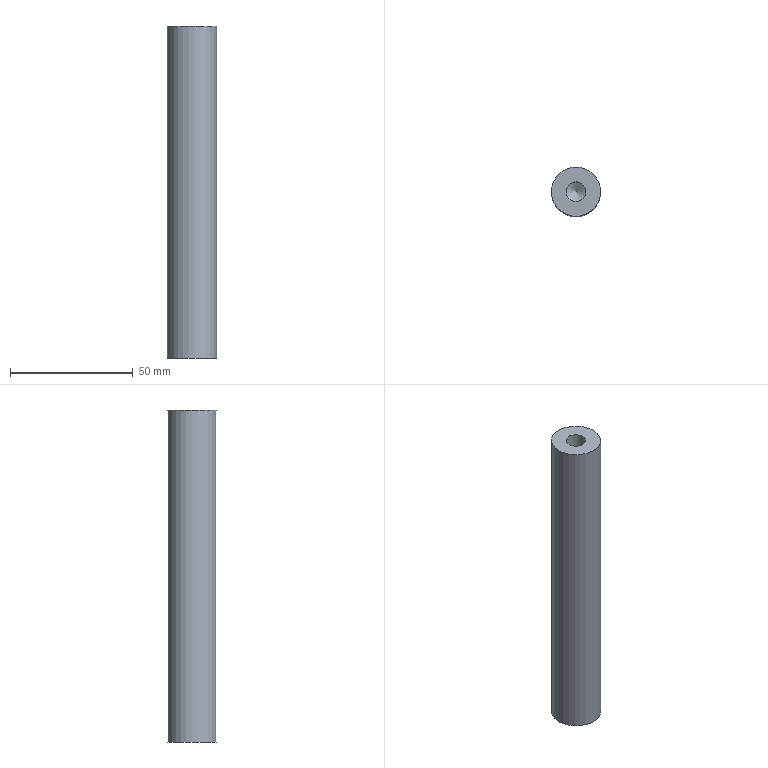Part | NX | features solid 2 | 1 solid | 7 faces | box 20 x 20 x 135 mm | volume 38516 mm3 | cylinder 3 | plane 2 | cone 2 | commonest cylinder face diameters 8 x1 12 x1 20 x1
STEP:
#1=CARTESIAN_POINT('',(-10.,175.,-155.));
#2=VERTEX_POINT('',#1);
#3=CARTESIAN_POINT('',(0.,175.,-155.));
#4=DIRECTION('',(0.,0.,-1.));
#5=DIRECTION('',(-1.,0.,0.));
#6=AXIS2_PLACEMENT_3D('',#3,#4,#5);
#7=CIRCLE('',#6,10.);
#8=EDGE_CURVE('',#2,#2,#7,.T.);
#9=ORIENTED_EDGE('',*,*,#8,.F.);
#10=EDGE_LOOP('',(#9));
#11=FACE_BOUND('',#10,.T.);
#12=CARTESIAN_POINT('',(10.,175.,-20.));
#13=VERTEX_POINT('',#12);
#14=CARTESIAN_POINT('',(0.,175.,-20.));
#15=DIRECTION('',(0.,0.,1.));
#16=DIRECTION('',(1.,0.,0.));
#17=AXIS2_PLACEMENT_3D('',#14,#15,#16);
#18=CIRCLE('',#17,10.);
#19=EDGE_CURVE('',#13,#13,#18,.F.);
#20=ORIENTED_EDGE('',*,*,#19,.T.);
#21=EDGE_LOOP('',(#20));
#22=FACE_BOUND('',#21,.T.);
#23=CARTESIAN_POINT('',(0.,175.,-97.));
#24=DIRECTION('',(0.,0.,1.));
#25=DIRECTION('',(0.,1.,0.));
#26=AXIS2_PLACEMENT_3D('',#23,#24,#25);
#27=CYLINDRICAL_SURFACE('',#26,10.);
#28=ADVANCED_FACE('',(#11,#22),#27,.T.);
#29=CARTESIAN_POINT('',(-6.,175.,-155.));
#30=VERTEX_POINT('',#29);
#31=CARTESIAN_POINT('',(0.,175.,-155.));
#32=DIRECTION('',(0.,0.,1.));
#33=DIRECTION('',(-1.,0.,0.));
#34=AXIS2_PLACEMENT_3D('',#31,#32,#33);
#35=CIRCLE('',#34,6.);
#36=EDGE_CURVE('',#30,#30,#35,.T.);
#37=ORIENTED_EDGE('',*,*,#36,.T.);
#38=EDGE_LOOP('',(#37));
#39=FACE_BOUND('',#38,.T.);
#40=ORIENTED_EDGE('',*,*,#8,.T.);
#41=EDGE_LOOP('',(#40));
#42=FACE_BOUND('',#41,.T.);
#43=CARTESIAN_POINT('',(0.,175.,-155.));
#44=DIRECTION('',(0.,0.,-1.));
#45=DIRECTION('',(0.,-1.,0.));
#46=AXIS2_PLACEMENT_3D('',#43,#44,#45);
#47=PLANE('',#46);
#48=ADVANCED_FACE('',(#39,#42),#47,.T.);
#49=CARTESIAN_POINT('',(-6.,175.,-131.));
#50=VERTEX_POINT('',#49);
#51=CARTESIAN_POINT('',(0.,175.,-131.));
#52=DIRECTION('',(0.,0.,1.));
#53=DIRECTION('',(-1.,0.,0.));
#54=AXIS2_PLACEMENT_3D('',#51,#52,#53);
#55=CIRCLE('',#54,6.);
#56=EDGE_CURVE('',#50,#50,#55,.T.);
#57=ORIENTED_EDGE('',*,*,#56,.F.);
#58=EDGE_LOOP('',(#57));
#59=FACE_BOUND('',#58,.T.);
#60=CARTESIAN_POINT('',(0.,175.,-127.395));
#61=VERTEX_POINT('',#60);
#62=VERTEX_LOOP('',#61);
#63=FACE_BOUND('',#62,.T.);
#64=CARTESIAN_POINT('',(0.,175.,-131.));
#65=DIRECTION('',(0.,0.,-1.));
#66=DIRECTION('',(1.,0.,0.));
#67=AXIS2_PLACEMENT_3D('',#64,#65,#66);
#68=CONICAL_SURFACE('',#67,6.,1.03);
#69=ADVANCED_FACE('',(#59,#63),#68,.F.);
#70=ORIENTED_EDGE('',*,*,#56,.T.);
#71=EDGE_LOOP('',(#70));
#72=FACE_BOUND('',#71,.T.);
#73=ORIENTED_EDGE('',*,*,#36,.F.);
#74=EDGE_LOOP('',(#73));
#75=FACE_BOUND('',#74,.T.);
#76=CARTESIAN_POINT('',(0.,175.,-145.));
#77=DIRECTION('',(0.,0.,1.));
#78=DIRECTION('',(-1.,0.,0.));
#79=AXIS2_PLACEMENT_3D('',#76,#77,#78);
#80=CYLINDRICAL_SURFACE('',#79,6.);
#81=ADVANCED_FACE('',(#72,#75),#80,.F.);
#82=CARTESIAN_POINT('',(-4.,175.,-20.));
#83=VERTEX_POINT('',#82);
#84=CARTESIAN_POINT('',(0.,175.,-20.));
#85=DIRECTION('',(0.,0.,-1.));
#86=DIRECTION('',(-1.,0.,0.));
#87=AXIS2_PLACEMENT_3D('',#84,#85,#86);
#88=CIRCLE('',#87,4.);
#89=EDGE_CURVE('',#83,#83,#88,.T.);
#90=ORIENTED_EDGE('',*,*,#89,.T.);
#91=EDGE_LOOP('',(#90));
#92=FACE_BOUND('',#91,.T.);
#93=ORIENTED_EDGE('',*,*,#19,.F.);
#94=EDGE_LOOP('',(#93));
#95=FACE_BOUND('',#94,.T.);
#96=CARTESIAN_POINT('',(0.,175.,-20.));
#97=DIRECTION('',(0.,0.,1.));
#98=DIRECTION('',(1.,0.,0.));
#99=AXIS2_PLACEMENT_3D('',#96,#97,#98);
#100=PLANE('',#99);
#101=ADVANCED_FACE('',(#92,#95),#100,.T.);
#102=CARTESIAN_POINT('',(-4.,175.,-40.));
#103=VERTEX_POINT('',#102);
#104=CARTESIAN_POINT('',(0.,175.,-40.));
#105=DIRECTION('',(0.,0.,-1.));
#106=DIRECTION('',(-1.,0.,0.));
#107=AXIS2_PLACEMENT_3D('',#104,#105,#106);
#108=CIRCLE('',#107,4.);
#109=EDGE_CURVE('',#103,#103,#108,.T.);
#110=ORIENTED_EDGE('',*,*,#109,.F.);
#111=EDGE_LOOP('',(#110));
#112=FACE_BOUND('',#111,.T.);
#113=CARTESIAN_POINT('',(0.,175.,-42.403));
#114=VERTEX_POINT('',#113);
#115=VERTEX_LOOP('',#114);
#116=FACE_BOUND('',#115,.T.);
#117=CARTESIAN_POINT('',(0.,175.,-40.));
#118=DIRECTION('',(0.,0.,1.));
#119=DIRECTION('',(1.,0.,0.));
#120=AXIS2_PLACEMENT_3D('',#117,#118,#119);
#121=CONICAL_SURFACE('',#120,4.,1.03);
#122=ADVANCED_FACE('',(#112,#116),#121,.F.);
#123=ORIENTED_EDGE('',*,*,#109,.T.);
#124=EDGE_LOOP('',(#123));
#125=FACE_BOUND('',#124,.T.);
#126=ORIENTED_EDGE('',*,*,#89,.F.);
#127=EDGE_LOOP('',(#126));
#128=FACE_BOUND('',#127,.T.);
#129=CARTESIAN_POINT('',(0.,175.,-20.));
#130=DIRECTION('',(0.,0.,-1.));
#131=DIRECTION('',(-1.,0.,0.));
#132=AXIS2_PLACEMENT_3D('',#129,#130,#131);
#133=CYLINDRICAL_SURFACE('',#132,4.);
#134=ADVANCED_FACE('',(#125,#128),#133,.F.);
#135=CLOSED_SHELL('',(#28,#48,#69,#81,#101,#122,#134));
#136=MANIFOLD_SOLID_BREP('',#135);
#137=(LENGTH_UNIT()NAMED_UNIT(*)SI_UNIT(.MILLI.,.METRE.));
#138=UNCERTAINTY_MEASURE_WITH_UNIT(LENGTH_MEASURE(0.00001),#137,'','');
#139=(NAMED_UNIT(*)PLANE_ANGLE_UNIT()SI_UNIT($,.RADIAN.));
#140=(NAMED_UNIT(*)SI_UNIT($,.STERADIAN.)SOLID_ANGLE_UNIT());
#141=(GEOMETRIC_REPRESENTATION_CONTEXT(3)GLOBAL_UNCERTAINTY_ASSIGNED_CONTEXT((#138))GLOBAL_UNIT_ASSIGNED_CONTEXT((#137,#139,#140))REPRESENTATION_CONTEXT('',''));
#142=ADVANCED_BREP_SHAPE_REPRESENTATION('',(#136),#141);